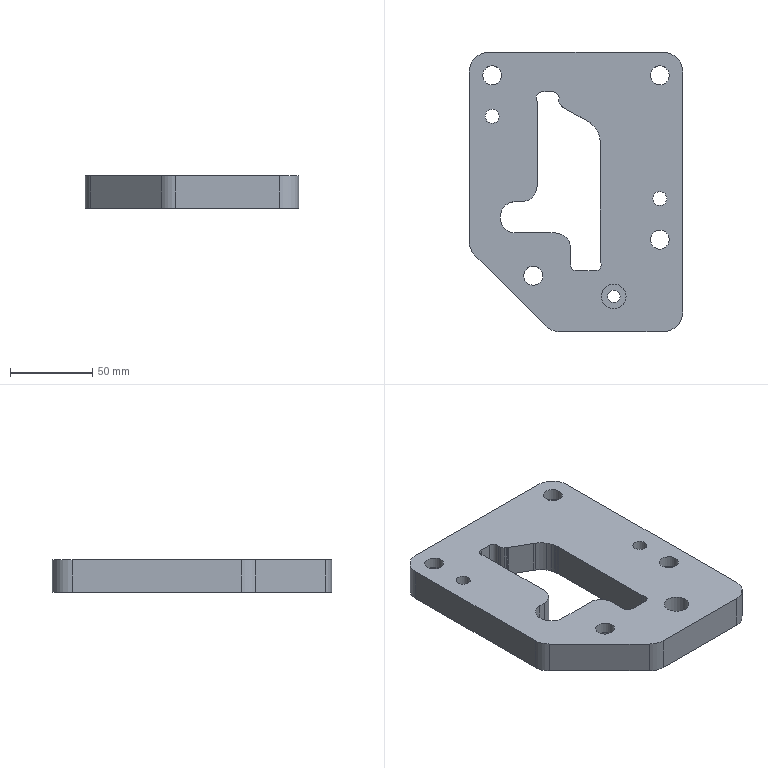Part | STEP file | lll_id98_x_t | 1 solid | 64 faces | box 130 x 170 x 20 mm | volume 318306 mm3 | cylinder 41 | plane 23 | commonest cylinder face diameters 24 x5 7 x4 11.509 x4 18.008 x4 5 x3 8.505 x2